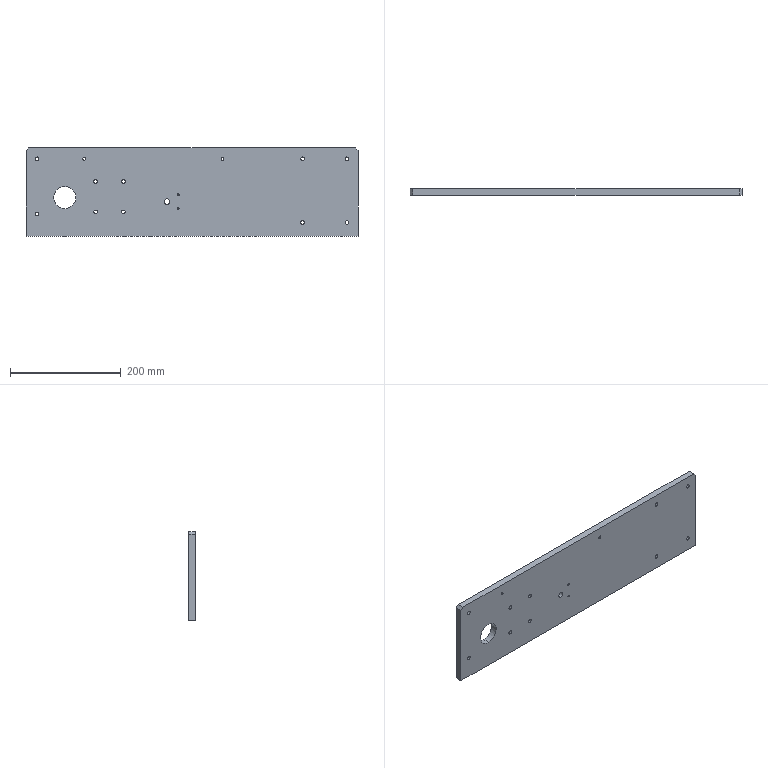Part | SolidWorks | features 3DProfileFeature 5, HoleWzd 5, Cut 2, Chamfer 1, Extrusion 1 | 1 solid | 70 faces | box 600 x 12 x 160 mm | volume 1127973 mm3 | cylinder 50 | plane 14 | cone 6 | commonest cylinder face diameters 6.6 x12 11 x12 3.3 x10 6.8 x8 5 x4 10 x2